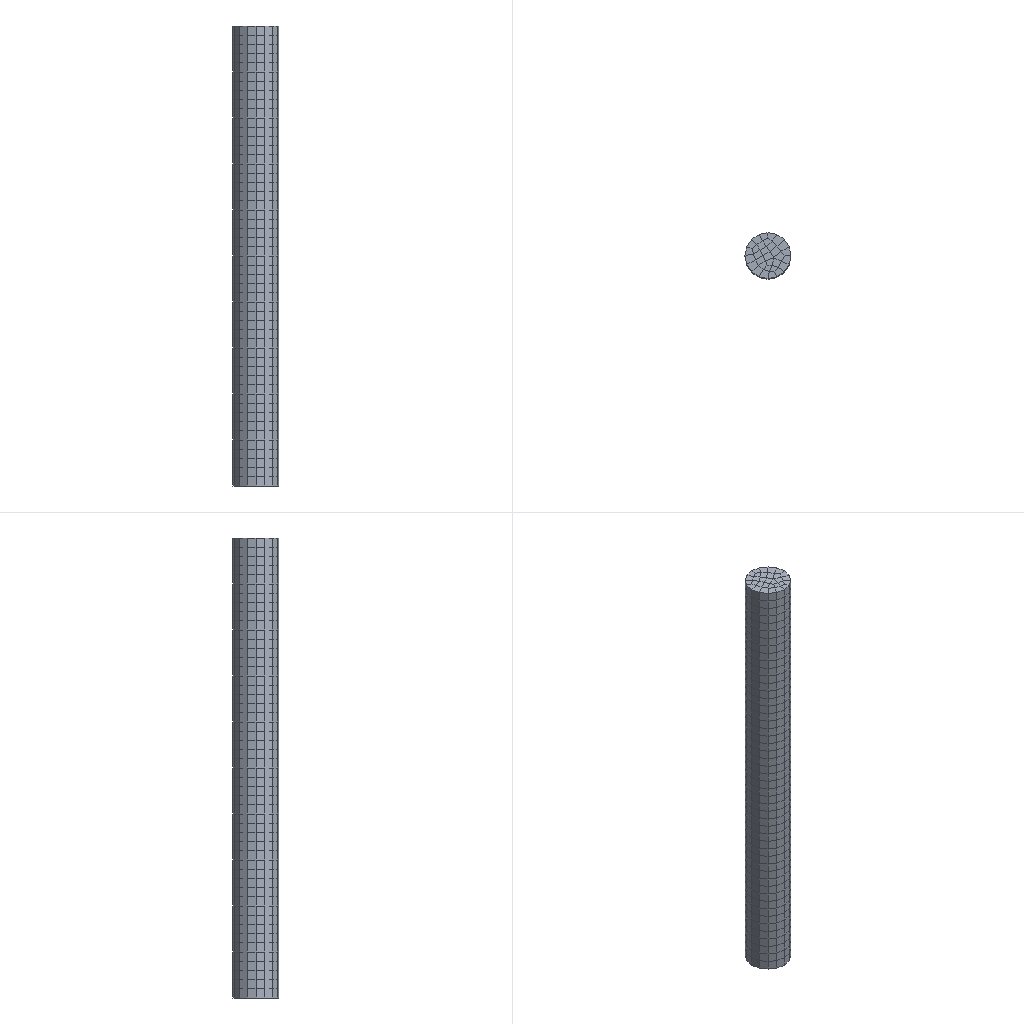Simulation study | abaqus
Set-up summary:
category,name,step,type,value,unit,region
solver,abaqus,,Abaqus/CAE 2024
units,unstated,,unstated,E=1 density= (no match)
analysis,Step-1,,static,time_period=1
mesh,nodes,,,2740
mesh,elements,,,2236
element_type,C3D8,,,1550
element_type,SFM3D4,,,686
material,pile,,E,1
material,pile,,nu,0
material,rebar,,E,2e+08
material,rebar,,nu,0
section,pile,,solid section,,,_PickedSet2
bc,BC-1,initial,fixed,"[dofs=x,y,z n=3]",,_PickedSet8
bc,BC-2,Step-1,displacement,-0.1 [dofs=z],,_PickedSet9
constraint,embedded element,,,1
Abaqus input file, long lists of numbers shortened:
*Heading
** Job name: deck Model name: Model-1
** Generated by: Abaqus/CAE 2024
*Preprint, echo=NO, model=NO, history=NO, contact=NO
**
** PARTS
**
*Part, name=pile
*Node
      1,  0.4619,  0.1913,           0.
      2,  0.1913,  0.4619,           0.
** (2038 more lines like these left out)
*Element, type=C3D8
   1,   56,   50,   58,   66,   16,   10,   18,   26
   2,   74,   58,   50,   49,   34,   18,   10,    9
** (1548 more lines like these left out)
*Nset, nset=_PickedSet2, internal, generate
    1,  2040,     1
*Elset, elset=_PickedSet2, internal, generate
    1,  1550,     1
*Nset, nset=pile, generate
    1,  2040,     1
*Elset, elset=pile, generate
    1,  1550,     1
** Section: pile
*Solid Section, elset=_PickedSet2, material=pile
,
*End Part
**
*Part, name=rebar
*Node
      1,  0.45,           0.,           0.
      2,  0.45,           0.,   0.2041
** (698 more lines like these left out)
*Element, type=SFM3D4
  1,   1,   2,  52,  51
  2,   2,   3,  53,  52
** (684 more lines like these left out)
*Nset, nset=_PickedSet2, internal, generate
   1,  700,    1
*Elset, elset=_PickedSet2, internal, generate
   1,  686,    1
*Nset, nset=rebar, generate
   1,  700,    1
*Elset, elset=rebar, generate
   1,  686,    1
** Section: rebar
*Surface Section, elset=_PickedSet2
*Rebar Layer
rebar-1, 1., 0.3533, , rebar, 90., 1
*End Part
**
**
** ASSEMBLY
**
*Assembly, name=Assembly
**
*Instance, name=pile-1, part=pile
*End Instance
**
*Instance, name=rebar-1, part=rebar
*End Instance
**
*Nset, nset=_PickedSet8, internal, instance=pile-1, generate
  1,  40,   1
*Elset, elset=_PickedSet8, internal, instance=pile-1, generate
  1,  31,   1
*Nset, nset=_PickedSet9, internal, instance=pile-1, generate
 2001,  2040,     1
*Elset, elset=_PickedSet9, internal, instance=pile-1, generate
 1520,  1550,     1
** Constraint: Constraint-1
*Embedded Element, host elset=pile-1.pile
rebar-1.rebar
*End Assembly
**
** MATERIALS
**
*Material, name=pile
*Elastic
1.,0.
*Material, name=rebar
*Elastic
 2e+08,0.
**
** BOUNDARY CONDITIONS
**
** Name: BC-1 Type: Displacement/Rotation
*Boundary
_PickedSet8, 1, 1
_PickedSet8, 2, 2
_PickedSet8, 3, 3
** ----------------------------------------------------------------
**
** STEP: Step-1
**
*Step, name=Step-1, nlgeom=NO
*Static
1., 1., 1e-05, 1.
**
** BOUNDARY CONDITIONS
**
** Name: BC-2 Type: Displacement/Rotation
*Boundary
_PickedSet9, 3, 3, -0.1
**
** OUTPUT REQUESTS
**
*Restart, write, frequency=0
**
** FIELD OUTPUT: F-Output-1
**
*Output, field
*Node Output
CF, RF, U
*Element Output, directions=YES
LE, PE, PEEQ, PEMAG, S
*Element Output, rebar, directions=YES
LE, PE, PEEQ, PEMAG, RBFOR, S
*Contact Output
CDISP, CSTRESS
**
** HISTORY OUTPUT: H-Output-1
**
*Output, history, variable=PRESELECT
*End Step
Results summary:
result,odb.job_status,,,JOB_STATUS_COMPLETED_SUCCESSFULLY,"consistent, unstated (Abaqus has no unit system)"
result,steps[0].procedure,Step-1,,*STATIC,"consistent, unstated (Abaqus has no unit system)"
result,steps[0].time_period,Step-1,,1,"consistent, unstated (Abaqus has no unit system)"
result,steps[0].n_frames,Step-1,,2,"consistent, unstated (Abaqus has no unit system)"
result,steps[0].last_frame.id,Step-1,,1,"consistent, unstated (Abaqus has no unit system)"
result,steps[0].last_frame.value,Step-1,,1,"consistent, unstated (Abaqus has no unit system)"
result,steps[0].last_frame.description,Step-1,,Increment      1: Step Time =    1.000,"consistent, unstated (Abaqus has no unit system)"
result,steps[0].completed,Step-1,,True,"consistent, unstated (Abaqus has no unit system)"
result,steps[0].max_U_magnitude,Step-1,,0.1,"consistent, unstated (Abaqus has no unit system)"
result,steps[0].max_S_mises,Step-1,,2e+06,"consistent, unstated (Abaqus has no unit system)"
result,steps[0].RF_sum[1],Step-1,,8.60423e-16,"consistent, unstated (Abaqus has no unit system)"
result,steps[0].RF_sum[2],Step-1,,-2.1684e-15,"consistent, unstated (Abaqus has no unit system)"
result,steps[0].RF_sum[3],Step-1,,1.187,"consistent, unstated (Abaqus has no unit system)"